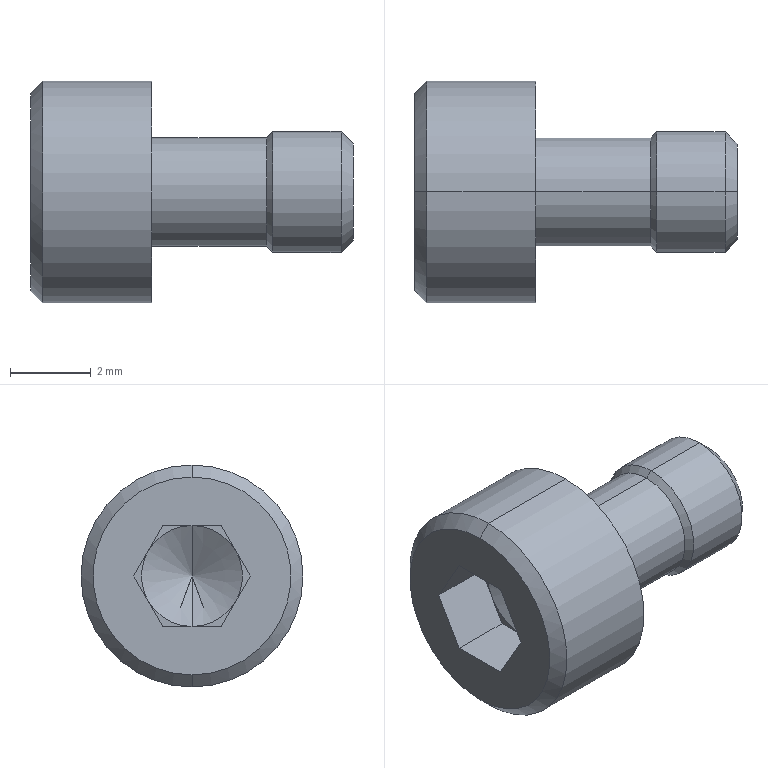Part | STEP file | 0243_Z_SCBS3-5_1 | 1 solid | 29 faces | box 8 x 5.5 x 5.5 mm | volume 92.14 mm3 | plane 15 | cone 8 | cylinder 6 | commonest cylinder face diameters 2.693 x2 3 x2 5.5 x2